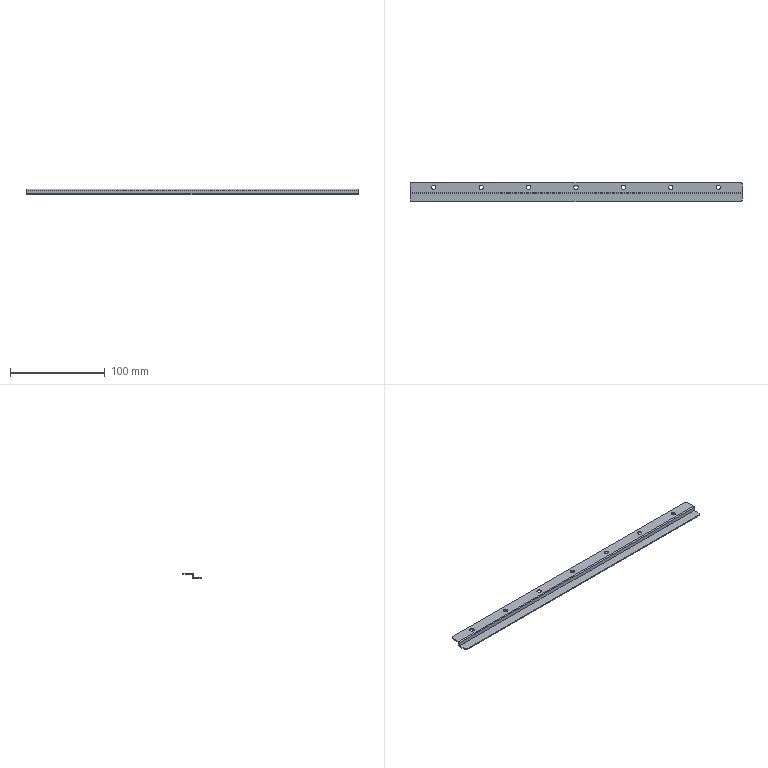Part | STEP file | 1 solid | 40 faces | box 350 x 21 x 6 mm | volume 8832 mm3 | cylinder 22 | plane 18 | commonest cylinder face diameters 4.5 x14 4 x4 0.02 x2 2.02 x2